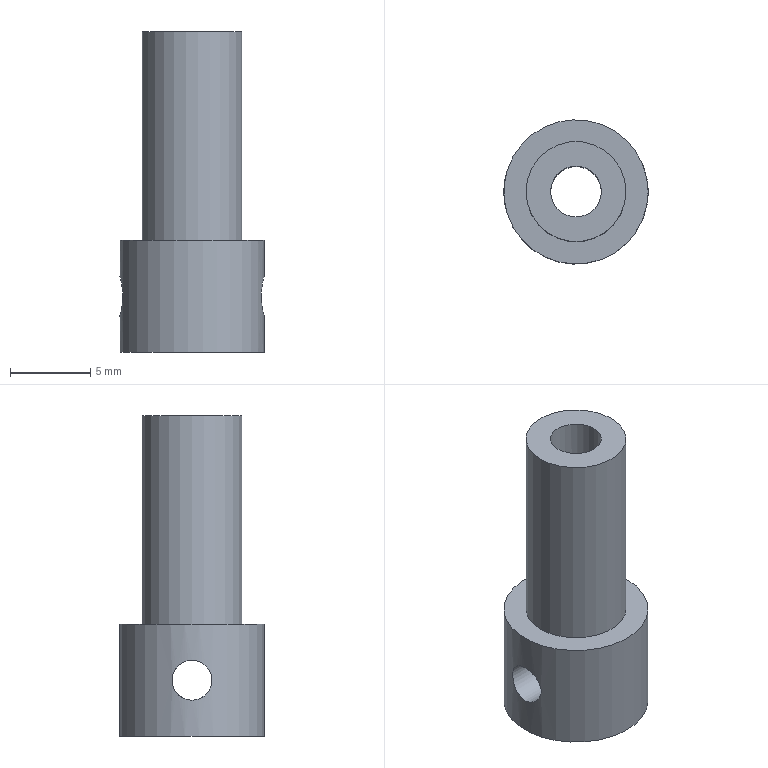Part | NX | features BREP 1, DATUM_CSYS 1 | 1 solid | 8 faces | box 9 x 9 x 20 mm | volume 655.524 mm3 | cylinder 5 | plane 3 | commonest cylinder face diameters 2.5 x2 3.17 x1 6.24 x1 9 x1
STEP:
#1=CARTESIAN_POINT('',(4.5,0.,0.));
#2=VERTEX_POINT('',#1);
#3=CARTESIAN_POINT('',(0.,0.,0.));
#4=DIRECTION('',(0.,0.,1.));
#5=DIRECTION('',(1.,0.,0.));
#6=AXIS2_PLACEMENT_3D('',#3,#4,#5);
#7=CIRCLE('',#6,4.5);
#8=EDGE_CURVE('',#2,#2,#7,.T.);
#9=ORIENTED_EDGE('',*,*,#8,.F.);
#10=EDGE_LOOP('',(#9));
#11=FACE_BOUND('',#10,.T.);
#12=CARTESIAN_POINT('',(1.585,0.,0.));
#13=VERTEX_POINT('',#12);
#14=CARTESIAN_POINT('',(0.,0.,0.));
#15=DIRECTION('',(0.,0.,-1.));
#16=DIRECTION('',(1.,0.,0.));
#17=AXIS2_PLACEMENT_3D('',#14,#15,#16);
#18=CIRCLE('',#17,1.585);
#19=EDGE_CURVE('',#13,#13,#18,.T.);
#20=ORIENTED_EDGE('',*,*,#19,.F.);
#21=EDGE_LOOP('',(#20));
#22=FACE_BOUND('',#21,.T.);
#23=CARTESIAN_POINT('',(0.,0.,0.));
#24=DIRECTION('',(0.,0.,1.));
#25=DIRECTION('',(-1.,0.,0.));
#26=AXIS2_PLACEMENT_3D('',#23,#24,#25);
#27=PLANE('',#26);
#28=ADVANCED_FACE('',(#11,#22),#27,.F.);
#29=CARTESIAN_POINT('',(4.5,0.,7.));
#30=VERTEX_POINT('',#29);
#31=CARTESIAN_POINT('',(0.,0.,7.));
#32=DIRECTION('',(0.,0.,1.));
#33=DIRECTION('',(1.,0.,0.));
#34=AXIS2_PLACEMENT_3D('',#31,#32,#33);
#35=CIRCLE('',#34,4.5);
#36=EDGE_CURVE('',#30,#30,#35,.T.);
#37=ORIENTED_EDGE('',*,*,#36,.T.);
#38=EDGE_LOOP('',(#37));
#39=FACE_BOUND('',#38,.T.);
#40=CARTESIAN_POINT('',(3.12,0.,7.));
#41=VERTEX_POINT('',#40);
#42=CARTESIAN_POINT('',(0.,0.,7.));
#43=DIRECTION('',(0.,0.,1.));
#44=DIRECTION('',(1.,0.,0.));
#45=AXIS2_PLACEMENT_3D('',#42,#43,#44);
#46=CIRCLE('',#45,3.12);
#47=EDGE_CURVE('',#41,#41,#46,.T.);
#48=ORIENTED_EDGE('',*,*,#47,.F.);
#49=EDGE_LOOP('',(#48));
#50=FACE_BOUND('',#49,.T.);
#51=CARTESIAN_POINT('',(0.,0.,7.));
#52=DIRECTION('',(0.,0.,1.));
#53=DIRECTION('',(-1.,0.,0.));
#54=AXIS2_PLACEMENT_3D('',#51,#52,#53);
#55=PLANE('',#54);
#56=ADVANCED_FACE('',(#39,#50),#55,.T.);
#57=ORIENTED_EDGE('',*,*,#8,.T.);
#58=CARTESIAN_POINT('',(4.5,0.,2.25));
#59=VERTEX_POINT('',#58);
#60=CARTESIAN_POINT('',(4.5,0.,0.));
#61=DIRECTION('',(0.,0.,1.));
#62=VECTOR('',#61,1000.);
#63=LINE('',#60,#62);
#64=EDGE_CURVE('',#2,#59,#63,.T.);
#65=ORIENTED_EDGE('',*,*,#64,.T.);
#66=CARTESIAN_POINT('',(4.5,0.,4.75));
#67=VERTEX_POINT('',#66);
#68=CARTESIAN_POINT('',(4.5,0.,4.75));
#69=CARTESIAN_POINT('',(4.5,-0.332,4.75));
#70=CARTESIAN_POINT('',(4.413,-0.977,4.479));
#71=CARTESIAN_POINT('',(4.278,-1.386,3.502));
#72=CARTESIAN_POINT('',(4.413,-0.9776,2.521));
#73=CARTESIAN_POINT('',(4.5,-0.332,2.25));
#74=CARTESIAN_POINT('',(4.5,0.,2.25));
#75=B_SPLINE_CURVE_WITH_KNOTS('',3,(#68,#69,#70,#71,#72,#73,#74),.UNSPECIFIED.,.F.,.F.,(4,1,1,1,4),(0.,0.0009815,0.001963,0.002945,0.003926),.UNSPECIFIED.);
#76=EDGE_CURVE('',#67,#59,#75,.T.);
#77=ORIENTED_EDGE('',*,*,#76,.F.);
#78=CARTESIAN_POINT('',(4.5,0.,4.75));
#79=DIRECTION('',(0.,0.,1.));
#80=VECTOR('',#79,1000.);
#81=LINE('',#78,#80);
#82=EDGE_CURVE('',#67,#30,#81,.T.);
#83=ORIENTED_EDGE('',*,*,#82,.T.);
#84=ORIENTED_EDGE('',*,*,#36,.F.);
#85=ORIENTED_EDGE('',*,*,#82,.F.);
#86=CARTESIAN_POINT('',(4.5,0.,2.25));
#87=CARTESIAN_POINT('',(4.5,0.332,2.25));
#88=CARTESIAN_POINT('',(4.413,0.977,2.521));
#89=CARTESIAN_POINT('',(4.278,1.386,3.498));
#90=CARTESIAN_POINT('',(4.413,0.9776,4.479));
#91=CARTESIAN_POINT('',(4.5,0.332,4.75));
#92=CARTESIAN_POINT('',(4.5,0.,4.75));
#93=B_SPLINE_CURVE_WITH_KNOTS('',3,(#86,#87,#88,#89,#90,#91,#92),.UNSPECIFIED.,.F.,.F.,(4,1,1,1,4),(0.,0.0009815,0.001963,0.002945,0.003926),.UNSPECIFIED.);
#94=EDGE_CURVE('',#59,#67,#93,.T.);
#95=ORIENTED_EDGE('',*,*,#94,.F.);
#96=ORIENTED_EDGE('',*,*,#64,.F.);
#97=EDGE_LOOP('',(#57,#65,#77,#83,#84,#85,#95,#96));
#98=FACE_BOUND('',#97,.T.);
#99=CARTESIAN_POINT('',(-4.5,0.,2.25));
#100=VERTEX_POINT('',#99);
#101=CARTESIAN_POINT('',(-4.413,0.9804,2.521));
#102=CARTESIAN_POINT('',(-4.543,-0.0001378,2.114));
#103=CARTESIAN_POINT('',(-4.413,-0.9798,2.521));
#104=CARTESIAN_POINT('',(-4.278,-1.385,3.498));
#105=CARTESIAN_POINT('',(-4.413,-0.9794,4.48));
#106=CARTESIAN_POINT('',(-4.543,-0.0006817,4.885));
#107=CARTESIAN_POINT('',(-4.413,0.9789,4.48));
#108=CARTESIAN_POINT('',(-4.278,1.385,3.5));
#109=CARTESIAN_POINT('',(-4.413,0.9804,2.521));
#110=CARTESIAN_POINT('',(-4.543,-0.0001378,2.114));
#111=CARTESIAN_POINT('',(-4.413,-0.9798,2.521));
#112=B_SPLINE_CURVE_WITH_KNOTS('',3,(#101,#102,#103,#104,#105,#106,#107,#108,#109,#110,#111),.UNSPECIFIED.,.T.,.F.,(1,1,1,1,1,1,1,1,1,1,1,1,1,1,1),(-0.002945,-0.001963,-0.0009817,0.,0.0009817,0.001963,0.002945,0.003927,0.004909,0.00589,0.006872,0.007854,0.008836,0.009817,0.0108),.UNSPECIFIED.);
#113=EDGE_CURVE('',#100,#100,#112,.T.);
#114=ORIENTED_EDGE('',*,*,#113,.F.);
#115=EDGE_LOOP('',(#114));
#116=FACE_BOUND('',#115,.T.);
#117=CARTESIAN_POINT('',(0.,0.,0.));
#118=DIRECTION('',(0.,0.,1.));
#119=DIRECTION('',(-1.,0.,0.));
#120=AXIS2_PLACEMENT_3D('',#117,#118,#119);
#121=CYLINDRICAL_SURFACE('',#120,4.5);
#122=ADVANCED_FACE('',(#98,#116),#121,.T.);
#123=ORIENTED_EDGE('',*,*,#47,.T.);
#124=CARTESIAN_POINT('',(3.12,0.,20.));
#125=VERTEX_POINT('',#124);
#126=CARTESIAN_POINT('',(3.12,0.,7.));
#127=DIRECTION('',(0.,0.,1.));
#128=VECTOR('',#127,1000.);
#129=LINE('',#126,#128);
#130=EDGE_CURVE('',#41,#125,#129,.T.);
#131=ORIENTED_EDGE('',*,*,#130,.T.);
#132=CARTESIAN_POINT('',(0.,0.,20.));
#133=DIRECTION('',(0.,0.,1.));
#134=DIRECTION('',(1.,0.,0.));
#135=AXIS2_PLACEMENT_3D('',#132,#133,#134);
#136=CIRCLE('',#135,3.12);
#137=EDGE_CURVE('',#125,#125,#136,.T.);
#138=ORIENTED_EDGE('',*,*,#137,.F.);
#139=ORIENTED_EDGE('',*,*,#130,.F.);
#140=EDGE_LOOP('',(#123,#131,#138,#139));
#141=FACE_BOUND('',#140,.T.);
#142=CARTESIAN_POINT('',(0.,0.,7.));
#143=DIRECTION('',(0.,0.,1.));
#144=DIRECTION('',(-1.,0.,0.));
#145=AXIS2_PLACEMENT_3D('',#142,#143,#144);
#146=CYLINDRICAL_SURFACE('',#145,3.12);
#147=ADVANCED_FACE('',(#141),#146,.T.);
#148=ORIENTED_EDGE('',*,*,#137,.T.);
#149=EDGE_LOOP('',(#148));
#150=FACE_BOUND('',#149,.T.);
#151=CARTESIAN_POINT('',(1.585,0.,20.));
#152=VERTEX_POINT('',#151);
#153=CARTESIAN_POINT('',(0.,0.,20.));
#154=DIRECTION('',(0.,0.,-1.));
#155=DIRECTION('',(1.,0.,0.));
#156=AXIS2_PLACEMENT_3D('',#153,#154,#155);
#157=CIRCLE('',#156,1.585);
#158=EDGE_CURVE('',#152,#152,#157,.T.);
#159=ORIENTED_EDGE('',*,*,#158,.T.);
#160=EDGE_LOOP('',(#159));
#161=FACE_BOUND('',#160,.T.);
#162=CARTESIAN_POINT('',(0.,0.,20.));
#163=DIRECTION('',(0.,0.,1.));
#164=DIRECTION('',(-1.,0.,0.));
#165=AXIS2_PLACEMENT_3D('',#162,#163,#164);
#166=PLANE('',#165);
#167=ADVANCED_FACE('',(#150,#161),#166,.T.);
#168=CARTESIAN_POINT('',(1.585,0.,4.75));
#169=VERTEX_POINT('',#168);
#170=CARTESIAN_POINT('',(1.585,0.,20.));
#171=DIRECTION('',(0.,0.,-1.));
#172=VECTOR('',#171,1000.);
#173=LINE('',#170,#172);
#174=EDGE_CURVE('',#152,#169,#173,.T.);
#175=ORIENTED_EDGE('',*,*,#174,.T.);
#176=CARTESIAN_POINT('',(1.585,0.,2.25));
#177=VERTEX_POINT('',#176);
#178=CARTESIAN_POINT('',(1.585,0.,2.25));
#179=CARTESIAN_POINT('',(1.585,-0.3497,2.25));
#180=CARTESIAN_POINT('',(1.343,-0.981,2.532));
#181=CARTESIAN_POINT('',(0.7907,-1.384,3.499));
#182=CARTESIAN_POINT('',(1.342,-0.9822,4.467));
#183=CARTESIAN_POINT('',(1.585,-0.3501,4.75));
#184=CARTESIAN_POINT('',(1.585,0.,4.75));
#185=B_SPLINE_CURVE_WITH_KNOTS('',3,(#178,#179,#180,#181,#182,#183,#184),.UNSPECIFIED.,.F.,.F.,(4,1,1,1,4),(0.,0.001032,0.002064,0.003095,0.004127),.UNSPECIFIED.);
#186=EDGE_CURVE('',#177,#169,#185,.T.);
#187=ORIENTED_EDGE('',*,*,#186,.F.);
#188=CARTESIAN_POINT('',(1.585,0.,2.25));
#189=DIRECTION('',(0.,0.,-1.));
#190=VECTOR('',#189,1000.);
#191=LINE('',#188,#190);
#192=EDGE_CURVE('',#177,#13,#191,.T.);
#193=ORIENTED_EDGE('',*,*,#192,.T.);
#194=ORIENTED_EDGE('',*,*,#19,.T.);
#195=ORIENTED_EDGE('',*,*,#192,.F.);
#196=CARTESIAN_POINT('',(1.585,0.,4.75));
#197=CARTESIAN_POINT('',(1.585,0.3497,4.75));
#198=CARTESIAN_POINT('',(1.343,0.981,4.468));
#199=CARTESIAN_POINT('',(0.7907,1.384,3.501));
#200=CARTESIAN_POINT('',(1.342,0.9822,2.533));
#201=CARTESIAN_POINT('',(1.585,0.3501,2.25));
#202=CARTESIAN_POINT('',(1.585,0.,2.25));
#203=B_SPLINE_CURVE_WITH_KNOTS('',3,(#196,#197,#198,#199,#200,#201,#202),.UNSPECIFIED.,.F.,.F.,(4,1,1,1,4),(0.,0.001032,0.002064,0.003095,0.004127),.UNSPECIFIED.);
#204=EDGE_CURVE('',#169,#177,#203,.T.);
#205=ORIENTED_EDGE('',*,*,#204,.F.);
#206=ORIENTED_EDGE('',*,*,#174,.F.);
#207=ORIENTED_EDGE('',*,*,#158,.F.);
#208=EDGE_LOOP('',(#175,#187,#193,#194,#195,#205,#206,#207));
#209=FACE_BOUND('',#208,.T.);
#210=CARTESIAN_POINT('',(-1.585,0.,2.25));
#211=VERTEX_POINT('',#210);
#212=CARTESIAN_POINT('',(-1.342,-0.9926,2.533));
#213=CARTESIAN_POINT('',(-1.706,0.0007381,2.109));
#214=CARTESIAN_POINT('',(-1.343,0.9896,2.532));
#215=CARTESIAN_POINT('',(-0.791,1.379,3.497));
#216=CARTESIAN_POINT('',(-1.34,0.9928,4.465));
#217=CARTESIAN_POINT('',(-1.706,0.007102,4.891));
#218=CARTESIAN_POINT('',(-1.344,-0.99,4.471));
#219=CARTESIAN_POINT('',(-0.7903,-1.379,3.501));
#220=CARTESIAN_POINT('',(-1.342,-0.9926,2.533));
#221=CARTESIAN_POINT('',(-1.706,0.0007381,2.109));
#222=CARTESIAN_POINT('',(-1.343,0.9896,2.532));
#223=B_SPLINE_CURVE_WITH_KNOTS('',3,(#212,#213,#214,#215,#216,#217,#218,#219,#220,#221,#222),.UNSPECIFIED.,.T.,.F.,(1,1,1,1,1,1,1,1,1,1,1,1,1,1,1),(-0.003093,-0.002062,-0.001031,0.,0.001031,0.002062,0.003093,0.004123,0.005154,0.006185,0.007216,0.008247,0.009278,0.01031,0.01134),.UNSPECIFIED.);
#224=EDGE_CURVE('',#211,#211,#223,.T.);
#225=ORIENTED_EDGE('',*,*,#224,.F.);
#226=EDGE_LOOP('',(#225));
#227=FACE_BOUND('',#226,.T.);
#228=CARTESIAN_POINT('',(0.,0.,20.));
#229=DIRECTION('',(0.,0.,-1.));
#230=DIRECTION('',(-1.,0.,0.));
#231=AXIS2_PLACEMENT_3D('',#228,#229,#230);
#232=CYLINDRICAL_SURFACE('',#231,1.585);
#233=ADVANCED_FACE('',(#209,#227),#232,.F.);
#234=CARTESIAN_POINT('',(4.5,0.,2.25));
#235=DIRECTION('',(-1.,0.,0.));
#236=VECTOR('',#235,1000.);
#237=LINE('',#234,#236);
#238=EDGE_CURVE('',#59,#177,#237,.T.);
#239=ORIENTED_EDGE('',*,*,#238,.T.);
#240=ORIENTED_EDGE('',*,*,#186,.T.);
#241=ORIENTED_EDGE('',*,*,#204,.T.);
#242=ORIENTED_EDGE('',*,*,#238,.F.);
#243=ORIENTED_EDGE('',*,*,#94,.T.);
#244=ORIENTED_EDGE('',*,*,#76,.T.);
#245=EDGE_LOOP('',(#239,#240,#241,#242,#243,#244));
#246=FACE_BOUND('',#245,.T.);
#247=CARTESIAN_POINT('',(4.5,0.,3.5));
#248=DIRECTION('',(-1.,0.,0.));
#249=DIRECTION('',(0.,0.,1.));
#250=AXIS2_PLACEMENT_3D('',#247,#248,#249);
#251=CYLINDRICAL_SURFACE('',#250,1.25);
#252=ADVANCED_FACE('',(#246),#251,.F.);
#253=CARTESIAN_POINT('',(-1.585,0.,2.25));
#254=DIRECTION('',(-1.,0.,0.));
#255=VECTOR('',#254,1000.);
#256=LINE('',#253,#255);
#257=EDGE_CURVE('',#211,#100,#256,.T.);
#258=ORIENTED_EDGE('',*,*,#257,.F.);
#259=ORIENTED_EDGE('',*,*,#224,.T.);
#260=ORIENTED_EDGE('',*,*,#257,.T.);
#261=ORIENTED_EDGE('',*,*,#113,.T.);
#262=EDGE_LOOP('',(#258,#259,#260,#261));
#263=FACE_BOUND('',#262,.T.);
#264=CARTESIAN_POINT('',(4.5,0.,3.5));
#265=DIRECTION('',(-1.,0.,0.));
#266=DIRECTION('',(0.,0.,1.));
#267=AXIS2_PLACEMENT_3D('',#264,#265,#266);
#268=CYLINDRICAL_SURFACE('',#267,1.25);
#269=ADVANCED_FACE('',(#263),#268,.F.);
#270=CLOSED_SHELL('',(#28,#56,#122,#147,#167,#233,#252,#269));
#271=MANIFOLD_SOLID_BREP('',#270);
#272=(LENGTH_UNIT()NAMED_UNIT(*)SI_UNIT(.MILLI.,.METRE.));
#273=UNCERTAINTY_MEASURE_WITH_UNIT(LENGTH_MEASURE(0.0508),#272,'','');
#274=(NAMED_UNIT(*)PLANE_ANGLE_UNIT()SI_UNIT($,.RADIAN.));
#275=(NAMED_UNIT(*)SI_UNIT($,.STERADIAN.)SOLID_ANGLE_UNIT());
#276=(GEOMETRIC_REPRESENTATION_CONTEXT(3)GLOBAL_UNCERTAINTY_ASSIGNED_CONTEXT((#273))GLOBAL_UNIT_ASSIGNED_CONTEXT((#272,#274,#275))REPRESENTATION_CONTEXT('',''));
#277=ADVANCED_BREP_SHAPE_REPRESENTATION('',(#271),#276);